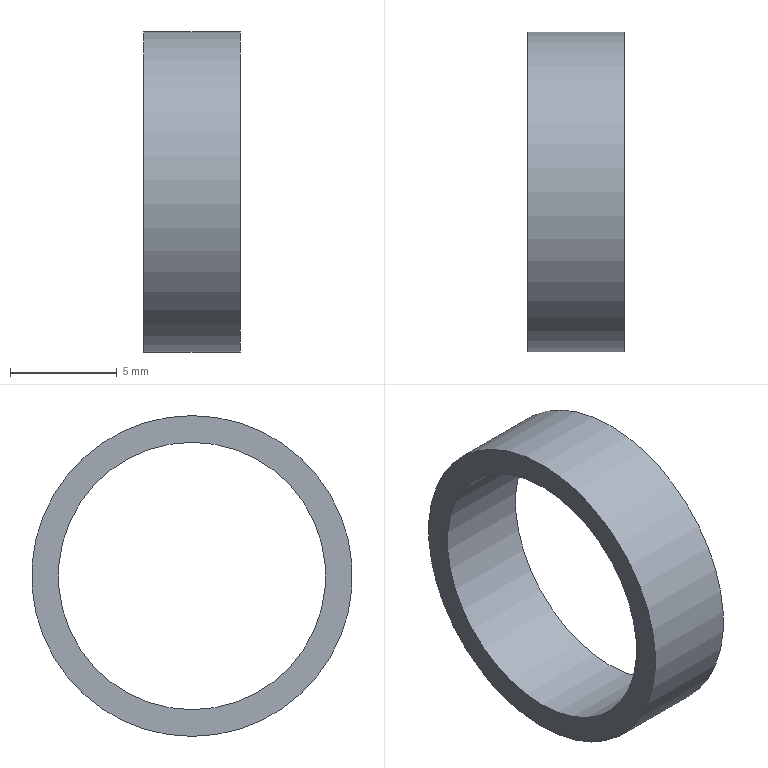Part | NX | 1 solid | 4 faces | box 4.5 x 15 x 15 mm | volume 242.983 mm3 | plane 2 | cylinder 2 | commonest cylinder face diameters 12.5 x1 15 x1
STEP:
#1=CARTESIAN_POINT('',(4.5,0.,-7.5));
#2=VERTEX_POINT('',#1);
#3=CARTESIAN_POINT('',(4.5,0.,0.));
#4=DIRECTION('',(1.,0.,0.));
#5=DIRECTION('',(0.,0.,-1.));
#6=AXIS2_PLACEMENT_3D('',#3,#4,#5);
#7=CIRCLE('',#6,7.5);
#8=EDGE_CURVE('',#2,#2,#7,.T.);
#9=ORIENTED_EDGE('',*,*,#8,.T.);
#10=EDGE_LOOP('',(#9));
#11=FACE_BOUND('',#10,.T.);
#12=CARTESIAN_POINT('',(4.5,0.,-6.25));
#13=VERTEX_POINT('',#12);
#14=CARTESIAN_POINT('',(4.5,0.,0.));
#15=DIRECTION('',(1.,0.,0.));
#16=DIRECTION('',(0.,0.,-1.));
#17=AXIS2_PLACEMENT_3D('',#14,#15,#16);
#18=CIRCLE('',#17,6.25);
#19=EDGE_CURVE('',#13,#13,#18,.T.);
#20=ORIENTED_EDGE('',*,*,#19,.F.);
#21=EDGE_LOOP('',(#20));
#22=FACE_BOUND('',#21,.T.);
#23=CARTESIAN_POINT('',(4.5,0.,0.));
#24=DIRECTION('',(1.,0.,0.));
#25=DIRECTION('',(0.,0.,-1.));
#26=AXIS2_PLACEMENT_3D('',#23,#24,#25);
#27=PLANE('',#26);
#28=ADVANCED_FACE('',(#11,#22),#27,.T.);
#29=CARTESIAN_POINT('',(0.,0.,-7.5));
#30=VERTEX_POINT('',#29);
#31=CARTESIAN_POINT('',(0.,0.,0.));
#32=DIRECTION('',(1.,0.,0.));
#33=DIRECTION('',(0.,0.,-1.));
#34=AXIS2_PLACEMENT_3D('',#31,#32,#33);
#35=CIRCLE('',#34,7.5);
#36=EDGE_CURVE('',#30,#30,#35,.T.);
#37=ORIENTED_EDGE('',*,*,#36,.F.);
#38=EDGE_LOOP('',(#37));
#39=FACE_BOUND('',#38,.T.);
#40=CARTESIAN_POINT('',(0.,0.,-6.25));
#41=VERTEX_POINT('',#40);
#42=CARTESIAN_POINT('',(0.,0.,0.));
#43=DIRECTION('',(1.,0.,0.));
#44=DIRECTION('',(0.,0.,-1.));
#45=AXIS2_PLACEMENT_3D('',#42,#43,#44);
#46=CIRCLE('',#45,6.25);
#47=EDGE_CURVE('',#41,#41,#46,.T.);
#48=ORIENTED_EDGE('',*,*,#47,.T.);
#49=EDGE_LOOP('',(#48));
#50=FACE_BOUND('',#49,.T.);
#51=CARTESIAN_POINT('',(0.,0.,0.));
#52=DIRECTION('',(1.,0.,0.));
#53=DIRECTION('',(0.,0.,-1.));
#54=AXIS2_PLACEMENT_3D('',#51,#52,#53);
#55=PLANE('',#54);
#56=ADVANCED_FACE('',(#39,#50),#55,.F.);
#57=ORIENTED_EDGE('',*,*,#8,.F.);
#58=EDGE_LOOP('',(#57));
#59=FACE_BOUND('',#58,.T.);
#60=ORIENTED_EDGE('',*,*,#36,.T.);
#61=EDGE_LOOP('',(#60));
#62=FACE_BOUND('',#61,.T.);
#63=CARTESIAN_POINT('',(4.5,0.,0.));
#64=DIRECTION('',(-1.,0.,0.));
#65=DIRECTION('',(0.,0.,1.));
#66=AXIS2_PLACEMENT_3D('',#63,#64,#65);
#67=CYLINDRICAL_SURFACE('',#66,7.5);
#68=ADVANCED_FACE('',(#59,#62),#67,.T.);
#69=ORIENTED_EDGE('',*,*,#19,.T.);
#70=EDGE_LOOP('',(#69));
#71=FACE_BOUND('',#70,.T.);
#72=ORIENTED_EDGE('',*,*,#47,.F.);
#73=EDGE_LOOP('',(#72));
#74=FACE_BOUND('',#73,.T.);
#75=CARTESIAN_POINT('',(4.5,0.,0.));
#76=DIRECTION('',(-1.,0.,0.));
#77=DIRECTION('',(0.,0.,1.));
#78=AXIS2_PLACEMENT_3D('',#75,#76,#77);
#79=CYLINDRICAL_SURFACE('',#78,6.25);
#80=ADVANCED_FACE('',(#71,#74),#79,.F.);
#81=CLOSED_SHELL('',(#28,#56,#68,#80));
#82=MANIFOLD_SOLID_BREP('',#81);
#83=(LENGTH_UNIT()NAMED_UNIT(*)SI_UNIT(.MILLI.,.METRE.));
#84=UNCERTAINTY_MEASURE_WITH_UNIT(LENGTH_MEASURE(0.00001),#83,'','');
#85=(NAMED_UNIT(*)PLANE_ANGLE_UNIT()SI_UNIT($,.RADIAN.));
#86=(NAMED_UNIT(*)SI_UNIT($,.STERADIAN.)SOLID_ANGLE_UNIT());
#87=(GEOMETRIC_REPRESENTATION_CONTEXT(3)GLOBAL_UNCERTAINTY_ASSIGNED_CONTEXT((#84))GLOBAL_UNIT_ASSIGNED_CONTEXT((#83,#85,#86))REPRESENTATION_CONTEXT('',''));
#88=ADVANCED_BREP_SHAPE_REPRESENTATION('',(#82),#87);